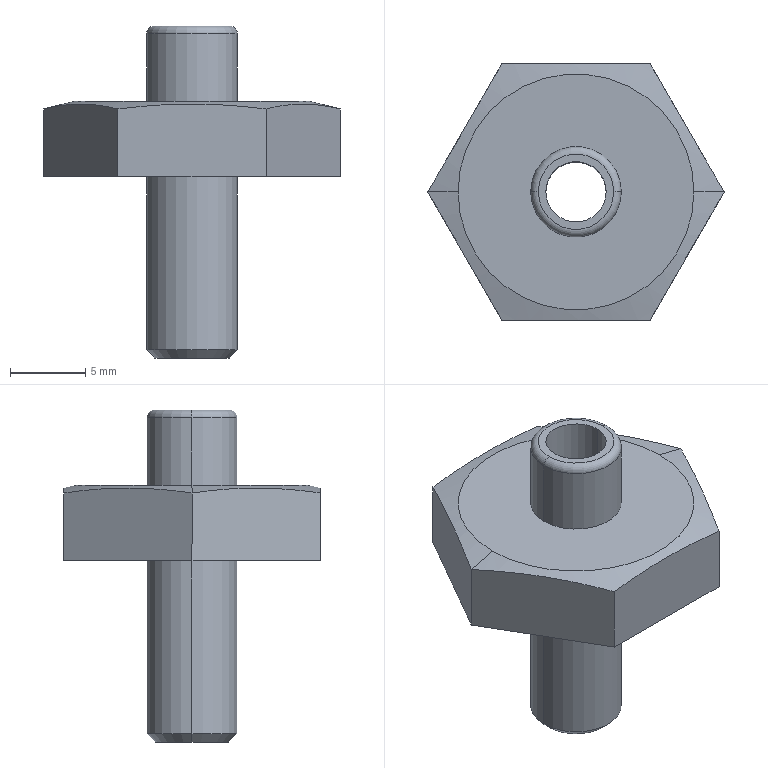Part | SolidWorks | features ICE 2, Cut 1, Extrusion 1, Fillet 1, RevCut 1, StudWizard 1 | 1 solid | 22 faces | box 19.63 x 17 x 22 mm | volume 1443 mm3 | plane 10 | cylinder 6 | cone 4 | torus 2 | commonest cylinder face diameters 6 x4 4 x2
STEP:
#1=CARTESIAN_POINT('',(-119.073,154.119,-12.));
#2=VERTEX_POINT('',#1);
#3=CARTESIAN_POINT('',(-123.99,154.119,-12.));
#4=VERTEX_POINT('',#3);
#5=CARTESIAN_POINT('',(-121.531,154.119,-12.));
#6=DIRECTION('',(0.,0.,1.));
#7=DIRECTION('',(1.,0.,0.));
#8=AXIS2_PLACEMENT_3D('',#5,#6,#7);
#9=CIRCLE('',#8,2.459);
#10=EDGE_CURVE('',#2,#4,#9,.T.);
#11=ORIENTED_EDGE('',*,*,#10,.T.);
#12=CARTESIAN_POINT('',(-124.531,154.119,-11.459));
#13=VERTEX_POINT('',#12);
#14=CARTESIAN_POINT('',(-123.99,154.119,-12.));
#15=DIRECTION('',(-0.7071,0.,0.7071));
#16=VECTOR('',#15,1000.);
#17=LINE('',#14,#16);
#18=EDGE_CURVE('',#4,#13,#17,.T.);
#19=ORIENTED_EDGE('',*,*,#18,.T.);
#20=CARTESIAN_POINT('',(-118.531,154.119,-11.459));
#21=VERTEX_POINT('',#20);
#22=CARTESIAN_POINT('',(-121.531,154.119,-11.459));
#23=DIRECTION('',(0.,0.,1.));
#24=DIRECTION('',(1.,0.,0.));
#25=AXIS2_PLACEMENT_3D('',#22,#23,#24);
#26=CIRCLE('',#25,3.);
#27=EDGE_CURVE('',#21,#13,#26,.T.);
#28=ORIENTED_EDGE('',*,*,#27,.F.);
#29=CARTESIAN_POINT('',(-119.073,154.119,-12.));
#30=DIRECTION('',(0.7071,0.,0.7071));
#31=VECTOR('',#30,1000.);
#32=LINE('',#29,#31);
#33=EDGE_CURVE('',#2,#21,#32,.T.);
#34=ORIENTED_EDGE('',*,*,#33,.F.);
#35=EDGE_LOOP('',(#11,#19,#28,#34));
#36=FACE_OUTER_BOUND('',#35,.T.);
#37=CARTESIAN_POINT('',(-121.531,154.119,-12.));
#38=DIRECTION('',(0.,0.,1.));
#39=DIRECTION('',(1.,0.,0.));
#40=AXIS2_PLACEMENT_3D('',#37,#38,#39);
#41=CONICAL_SURFACE('',#40,2.459,0.7854);
#42=ADVANCED_FACE('',(#36),#41,.T.);
#43=CARTESIAN_POINT('',(-124.531,154.119,9.5));
#44=VERTEX_POINT('',#43);
#45=CARTESIAN_POINT('',(-118.531,154.119,9.5));
#46=VERTEX_POINT('',#45);
#47=CARTESIAN_POINT('',(-121.531,154.119,9.5));
#48=DIRECTION('',(0.,0.,-1.));
#49=DIRECTION('',(1.,0.,0.));
#50=AXIS2_PLACEMENT_3D('',#47,#48,#49);
#51=CIRCLE('',#50,3.);
#52=EDGE_CURVE('',#44,#46,#51,.T.);
#53=ORIENTED_EDGE('',*,*,#52,.F.);
#54=CARTESIAN_POINT('',(-124.031,154.119,10.));
#55=VERTEX_POINT('',#54);
#56=CARTESIAN_POINT('',(-124.031,154.119,9.5));
#57=DIRECTION('',(0.,1.,0.));
#58=DIRECTION('',(-1.,0.,0.));
#59=AXIS2_PLACEMENT_3D('',#56,#57,#58);
#60=CIRCLE('',#59,0.5);
#61=EDGE_CURVE('',#44,#55,#60,.T.);
#62=ORIENTED_EDGE('',*,*,#61,.T.);
#63=CARTESIAN_POINT('',(-119.031,154.119,10.));
#64=VERTEX_POINT('',#63);
#65=CARTESIAN_POINT('',(-121.531,154.119,10.));
#66=DIRECTION('',(0.,0.,1.));
#67=DIRECTION('',(1.,0.,0.));
#68=AXIS2_PLACEMENT_3D('',#65,#66,#67);
#69=CIRCLE('',#68,2.5);
#70=EDGE_CURVE('',#64,#55,#69,.T.);
#71=ORIENTED_EDGE('',*,*,#70,.F.);
#72=CARTESIAN_POINT('',(-119.031,154.119,9.5));
#73=DIRECTION('',(0.,-1.,0.));
#74=DIRECTION('',(0.,0.,-1.));
#75=AXIS2_PLACEMENT_3D('',#72,#73,#74);
#76=CIRCLE('',#75,0.5);
#77=EDGE_CURVE('',#46,#64,#76,.T.);
#78=ORIENTED_EDGE('',*,*,#77,.F.);
#79=EDGE_LOOP('',(#53,#62,#71,#78));
#80=FACE_OUTER_BOUND('',#79,.T.);
#81=CARTESIAN_POINT('',(-121.531,154.119,9.5));
#82=DIRECTION('',(0.,0.,1.));
#83=DIRECTION('',(1.,0.,0.));
#84=AXIS2_PLACEMENT_3D('',#81,#82,#83);
#85=TOROIDAL_SURFACE('',#84,2.5,0.5);
#86=ADVANCED_FACE('',(#80),#85,.T.);
#87=CARTESIAN_POINT('',(-113.716,154.119,5.));
#88=VERTEX_POINT('',#87);
#89=CARTESIAN_POINT('',(-129.346,154.119,5.));
#90=VERTEX_POINT('',#89);
#91=CARTESIAN_POINT('',(-121.531,154.119,5.));
#92=DIRECTION('',(0.,0.,1.));
#93=DIRECTION('',(1.,0.,0.));
#94=AXIS2_PLACEMENT_3D('',#91,#92,#93);
#95=CIRCLE('',#94,7.815);
#96=EDGE_CURVE('',#88,#90,#95,.T.);
#97=ORIENTED_EDGE('',*,*,#96,.F.);
#98=CARTESIAN_POINT('',(-111.716,154.119,4.5));
#99=VERTEX_POINT('',#98);
#100=CARTESIAN_POINT('',(-111.716,154.119,4.5));
#101=DIRECTION('',(0.9701,0.,-0.2425));
#102=VECTOR('',#101,1000.);
#103=LINE('',#100,#102);
#104=EDGE_CURVE('',#88,#99,#103,.T.);
#105=ORIENTED_EDGE('',*,*,#104,.T.);
#106=CARTESIAN_POINT('',(-116.624,162.619,4.5));
#107=VERTEX_POINT('',#106);
#108=CARTESIAN_POINT('',(-116.624,162.619,4.5));
#109=CARTESIAN_POINT('',(-115.806,161.202,4.704));
#110=CARTESIAN_POINT('',(-114.17,158.369,4.953));
#111=CARTESIAN_POINT('',(-112.534,155.536,4.704));
#112=CARTESIAN_POINT('',(-111.716,154.119,4.5));
#113=B_SPLINE_CURVE_WITH_KNOTS('',3,(#108,#109,#110,#111,#112),.UNSPECIFIED.,.F.,.F.,(4,1,4),(0.000000231,0.004908,0.009815),.UNSPECIFIED.);
#114=EDGE_CURVE('',#107,#99,#113,.T.);
#115=ORIENTED_EDGE('',*,*,#114,.F.);
#116=CARTESIAN_POINT('',(-126.439,162.619,4.5));
#117=VERTEX_POINT('',#116);
#118=CARTESIAN_POINT('',(-126.439,162.619,4.5));
#119=CARTESIAN_POINT('',(-124.823,162.619,4.702));
#120=CARTESIAN_POINT('',(-123.199,162.619,4.827));
#121=CARTESIAN_POINT('',(-120.741,162.619,4.829));
#122=CARTESIAN_POINT('',(-119.918,162.619,4.8));
#123=CARTESIAN_POINT('',(-118.265,162.619,4.686));
#124=CARTESIAN_POINT('',(-117.443,162.619,4.602));
#125=CARTESIAN_POINT('',(-116.624,162.619,4.5));
#126=B_SPLINE_CURVE_WITH_KNOTS('',3,(#118,#119,#120,#121,#122,#123,#124,#125),.UNSPECIFIED.,.F.,.F.,(4,2,2,4),(0.009971,0.01485,0.0173,0.01974),.UNSPECIFIED.);
#127=EDGE_CURVE('',#117,#107,#126,.T.);
#128=ORIENTED_EDGE('',*,*,#127,.F.);
#129=CARTESIAN_POINT('',(-131.346,154.119,4.5));
#130=VERTEX_POINT('',#129);
#131=CARTESIAN_POINT('',(-131.346,154.119,4.5));
#132=CARTESIAN_POINT('',(-130.528,155.536,4.704));
#133=CARTESIAN_POINT('',(-128.892,158.369,4.953));
#134=CARTESIAN_POINT('',(-127.257,161.202,4.704));
#135=CARTESIAN_POINT('',(-126.439,162.619,4.5));
#136=B_SPLINE_CURVE_WITH_KNOTS('',3,(#131,#132,#133,#134,#135),.UNSPECIFIED.,.F.,.F.,(4,1,4),(0.000000231,0.004908,0.009815),.UNSPECIFIED.);
#137=EDGE_CURVE('',#130,#117,#136,.T.);
#138=ORIENTED_EDGE('',*,*,#137,.F.);
#139=CARTESIAN_POINT('',(-131.346,154.119,4.5));
#140=DIRECTION('',(-0.9701,0.,-0.2425));
#141=VECTOR('',#140,1000.);
#142=LINE('',#139,#141);
#143=EDGE_CURVE('',#90,#130,#142,.T.);
#144=ORIENTED_EDGE('',*,*,#143,.F.);
#145=EDGE_LOOP('',(#97,#105,#115,#128,#138,#144));
#146=FACE_OUTER_BOUND('',#145,.T.);
#147=CARTESIAN_POINT('',(-121.531,154.119,4.5));
#148=DIRECTION('',(0.,0.,-1.));
#149=DIRECTION('',(-1.,0.,0.));
#150=AXIS2_PLACEMENT_3D('',#147,#148,#149);
#151=CONICAL_SURFACE('',#150,9.815,1.326);
#152=ADVANCED_FACE('',(#146),#151,.T.);
#153=CARTESIAN_POINT('',(-119.531,154.119,-12.));
#154=VERTEX_POINT('',#153);
#155=CARTESIAN_POINT('',(-123.531,154.119,-12.));
#156=VERTEX_POINT('',#155);
#157=CARTESIAN_POINT('',(-121.531,154.119,-12.));
#158=DIRECTION('',(0.,0.,-1.));
#159=DIRECTION('',(-1.,0.,0.));
#160=AXIS2_PLACEMENT_3D('',#157,#158,#159);
#161=CIRCLE('',#160,2.);
#162=EDGE_CURVE('',#154,#156,#161,.T.);
#163=ORIENTED_EDGE('',*,*,#162,.T.);
#164=CARTESIAN_POINT('',(-123.531,154.119,10.));
#165=VERTEX_POINT('',#164);
#166=CARTESIAN_POINT('',(-123.531,154.119,-22.));
#167=DIRECTION('',(0.,0.,1.));
#168=VECTOR('',#167,1000.);
#169=LINE('',#166,#168);
#170=EDGE_CURVE('',#156,#165,#169,.T.);
#171=ORIENTED_EDGE('',*,*,#170,.T.);
#172=CARTESIAN_POINT('',(-119.531,154.119,10.));
#173=VERTEX_POINT('',#172);
#174=CARTESIAN_POINT('',(-121.531,154.119,10.));
#175=DIRECTION('',(0.,0.,1.));
#176=DIRECTION('',(1.,0.,0.));
#177=AXIS2_PLACEMENT_3D('',#174,#175,#176);
#178=CIRCLE('',#177,2.);
#179=EDGE_CURVE('',#165,#173,#178,.T.);
#180=ORIENTED_EDGE('',*,*,#179,.T.);
#181=CARTESIAN_POINT('',(-119.531,154.119,-22.));
#182=DIRECTION('',(0.,0.,1.));
#183=VECTOR('',#182,1000.);
#184=LINE('',#181,#183);
#185=EDGE_CURVE('',#154,#173,#184,.T.);
#186=ORIENTED_EDGE('',*,*,#185,.F.);
#187=EDGE_LOOP('',(#163,#171,#180,#186));
#188=FACE_OUTER_BOUND('',#187,.T.);
#189=CARTESIAN_POINT('',(-121.531,154.119,-22.));
#190=DIRECTION('',(0.,0.,1.));
#191=DIRECTION('',(1.,0.,0.));
#192=AXIS2_PLACEMENT_3D('',#189,#190,#191);
#193=CYLINDRICAL_SURFACE('',#192,2.);
#194=ADVANCED_FACE('',(#188),#193,.F.);
#195=ORIENTED_EDGE('',*,*,#27,.T.);
#196=CARTESIAN_POINT('',(-124.531,154.119,0.));
#197=VERTEX_POINT('',#196);
#198=CARTESIAN_POINT('',(-124.531,154.119,-12.));
#199=DIRECTION('',(0.,0.,1.));
#200=VECTOR('',#199,1000.);
#201=LINE('',#198,#200);
#202=EDGE_CURVE('',#13,#197,#201,.T.);
#203=ORIENTED_EDGE('',*,*,#202,.T.);
#204=CARTESIAN_POINT('',(-118.531,154.119,0.));
#205=VERTEX_POINT('',#204);
#206=CARTESIAN_POINT('',(-121.531,154.119,0.));
#207=DIRECTION('',(0.,0.,-1.));
#208=DIRECTION('',(-1.,0.,0.));
#209=AXIS2_PLACEMENT_3D('',#206,#207,#208);
#210=CIRCLE('',#209,3.);
#211=EDGE_CURVE('',#197,#205,#210,.T.);
#212=ORIENTED_EDGE('',*,*,#211,.T.);
#213=CARTESIAN_POINT('',(-118.531,154.119,-12.));
#214=DIRECTION('',(0.,0.,1.));
#215=VECTOR('',#214,1000.);
#216=LINE('',#213,#215);
#217=EDGE_CURVE('',#21,#205,#216,.T.);
#218=ORIENTED_EDGE('',*,*,#217,.F.);
#219=EDGE_LOOP('',(#195,#203,#212,#218));
#220=FACE_OUTER_BOUND('',#219,.T.);
#221=CARTESIAN_POINT('',(-121.531,154.119,-12.));
#222=DIRECTION('',(0.,0.,1.));
#223=DIRECTION('',(1.,0.,0.));
#224=AXIS2_PLACEMENT_3D('',#221,#222,#223);
#225=CYLINDRICAL_SURFACE('',#224,3.);
#226=ADVANCED_FACE('',(#220),#225,.T.);
#227=ORIENTED_EDGE('',*,*,#52,.T.);
#228=CARTESIAN_POINT('',(-118.531,154.119,5.));
#229=VERTEX_POINT('',#228);
#230=CARTESIAN_POINT('',(-118.531,154.119,10.));
#231=DIRECTION('',(0.,0.,-1.));
#232=VECTOR('',#231,1000.);
#233=LINE('',#230,#232);
#234=EDGE_CURVE('',#46,#229,#233,.T.);
#235=ORIENTED_EDGE('',*,*,#234,.T.);
#236=CARTESIAN_POINT('',(-124.531,154.119,5.));
#237=VERTEX_POINT('',#236);
#238=CARTESIAN_POINT('',(-121.531,154.119,5.));
#239=DIRECTION('',(0.,0.,1.));
#240=DIRECTION('',(1.,0.,0.));
#241=AXIS2_PLACEMENT_3D('',#238,#239,#240);
#242=CIRCLE('',#241,3.);
#243=EDGE_CURVE('',#229,#237,#242,.T.);
#244=ORIENTED_EDGE('',*,*,#243,.T.);
#245=CARTESIAN_POINT('',(-124.531,154.119,10.));
#246=DIRECTION('',(0.,0.,-1.));
#247=VECTOR('',#246,1000.);
#248=LINE('',#245,#247);
#249=EDGE_CURVE('',#44,#237,#248,.T.);
#250=ORIENTED_EDGE('',*,*,#249,.F.);
#251=EDGE_LOOP('',(#227,#235,#244,#250));
#252=FACE_OUTER_BOUND('',#251,.T.);
#253=CARTESIAN_POINT('',(-121.531,154.119,10.));
#254=DIRECTION('',(0.,0.,-1.));
#255=DIRECTION('',(-1.,0.,0.));
#256=AXIS2_PLACEMENT_3D('',#253,#254,#255);
#257=CYLINDRICAL_SURFACE('',#256,3.);
#258=ADVANCED_FACE('',(#252),#257,.T.);
#259=ORIENTED_EDGE('',*,*,#162,.F.);
#260=CARTESIAN_POINT('',(-121.531,154.119,-12.));
#261=DIRECTION('',(0.,0.,-1.));
#262=DIRECTION('',(-1.,0.,0.));
#263=AXIS2_PLACEMENT_3D('',#260,#261,#262);
#264=CIRCLE('',#263,2.);
#265=EDGE_CURVE('',#156,#154,#264,.T.);
#266=ORIENTED_EDGE('',*,*,#265,.F.);
#267=EDGE_LOOP('',(#259,#266));
#268=FACE_BOUND('',#267,.T.);
#269=ORIENTED_EDGE('',*,*,#10,.F.);
#270=CARTESIAN_POINT('',(-121.531,154.119,-12.));
#271=DIRECTION('',(0.,0.,1.));
#272=DIRECTION('',(1.,0.,0.));
#273=AXIS2_PLACEMENT_3D('',#270,#271,#272);
#274=CIRCLE('',#273,2.459);
#275=EDGE_CURVE('',#4,#2,#274,.T.);
#276=ORIENTED_EDGE('',*,*,#275,.F.);
#277=EDGE_LOOP('',(#269,#276));
#278=FACE_OUTER_BOUND('',#277,.T.);
#279=CARTESIAN_POINT('',(-121.531,154.119,-12.));
#280=DIRECTION('',(0.,0.,-1.));
#281=DIRECTION('',(-1.,0.,0.));
#282=AXIS2_PLACEMENT_3D('',#279,#280,#281);
#283=PLANE('',#282);
#284=ADVANCED_FACE('',(#268,#278),#283,.T.);
#285=CARTESIAN_POINT('',(-121.531,154.119,5.));
#286=DIRECTION('',(0.,0.,1.));
#287=DIRECTION('',(1.,0.,0.));
#288=AXIS2_PLACEMENT_3D('',#285,#286,#287);
#289=CIRCLE('',#288,3.);
#290=EDGE_CURVE('',#237,#229,#289,.T.);
#291=ORIENTED_EDGE('',*,*,#290,.F.);
#292=ORIENTED_EDGE('',*,*,#243,.F.);
#293=EDGE_LOOP('',(#291,#292));
#294=FACE_BOUND('',#293,.T.);
#295=CARTESIAN_POINT('',(-121.531,154.119,5.));
#296=DIRECTION('',(0.,0.,1.));
#297=DIRECTION('',(1.,0.,0.));
#298=AXIS2_PLACEMENT_3D('',#295,#296,#297);
#299=CIRCLE('',#298,7.815);
#300=EDGE_CURVE('',#90,#88,#299,.T.);
#301=ORIENTED_EDGE('',*,*,#300,.T.);
#302=ORIENTED_EDGE('',*,*,#96,.T.);
#303=EDGE_LOOP('',(#301,#302));
#304=FACE_OUTER_BOUND('',#303,.T.);
#305=CARTESIAN_POINT('',(0.,0.,5.));
#306=DIRECTION('',(0.,0.,1.));
#307=DIRECTION('',(1.,0.,0.));
#308=AXIS2_PLACEMENT_3D('',#305,#306,#307);
#309=PLANE('',#308);
#310=ADVANCED_FACE('',(#294,#304),#309,.T.);
#311=CARTESIAN_POINT('',(-116.624,162.619,0.));
#312=VERTEX_POINT('',#311);
#313=CARTESIAN_POINT('',(-116.624,162.619,5.));
#314=DIRECTION('',(0.,0.,-1.));
#315=VECTOR('',#314,1000.);
#316=LINE('',#313,#315);
#317=EDGE_CURVE('',#107,#312,#316,.T.);
#318=ORIENTED_EDGE('',*,*,#317,.F.);
#319=ORIENTED_EDGE('',*,*,#114,.T.);
#320=CARTESIAN_POINT('',(-111.716,154.119,0.));
#321=VERTEX_POINT('',#320);
#322=CARTESIAN_POINT('',(-111.716,154.119,5.));
#323=DIRECTION('',(0.,0.,-1.));
#324=VECTOR('',#323,1000.);
#325=LINE('',#322,#324);
#326=EDGE_CURVE('',#99,#321,#325,.T.);
#327=ORIENTED_EDGE('',*,*,#326,.T.);
#328=CARTESIAN_POINT('',(-111.716,154.119,0.));
#329=DIRECTION('',(-0.5,0.866,0.));
#330=VECTOR('',#329,1000.);
#331=LINE('',#328,#330);
#332=EDGE_CURVE('',#321,#312,#331,.T.);
#333=ORIENTED_EDGE('',*,*,#332,.T.);
#334=EDGE_LOOP('',(#318,#319,#327,#333));
#335=FACE_OUTER_BOUND('',#334,.T.);
#336=CARTESIAN_POINT('',(-111.716,154.119,5.));
#337=DIRECTION('',(-0.866,-0.5,0.));
#338=DIRECTION('',(0.5,-0.866,0.));
#339=AXIS2_PLACEMENT_3D('',#336,#337,#338);
#340=PLANE('',#339);
#341=ADVANCED_FACE('',(#335),#340,.F.);
#342=CARTESIAN_POINT('',(-126.439,162.619,0.));
#343=VERTEX_POINT('',#342);
#344=CARTESIAN_POINT('',(-126.439,162.619,5.));
#345=DIRECTION('',(0.,0.,-1.));
#346=VECTOR('',#345,1000.);
#347=LINE('',#344,#346);
#348=EDGE_CURVE('',#117,#343,#347,.T.);
#349=ORIENTED_EDGE('',*,*,#348,.F.);
#350=ORIENTED_EDGE('',*,*,#127,.T.);
#351=ORIENTED_EDGE('',*,*,#317,.T.);
#352=CARTESIAN_POINT('',(-116.624,162.619,0.));
#353=DIRECTION('',(-1.,0.,0.));
#354=VECTOR('',#353,1000.);
#355=LINE('',#352,#354);
#356=EDGE_CURVE('',#312,#343,#355,.T.);
#357=ORIENTED_EDGE('',*,*,#356,.T.);
#358=EDGE_LOOP('',(#349,#350,#351,#357));
#359=FACE_OUTER_BOUND('',#358,.T.);
#360=CARTESIAN_POINT('',(-116.624,162.619,5.));
#361=DIRECTION('',(0.,-1.,0.));
#362=DIRECTION('',(0.,0.,-1.));
#363=AXIS2_PLACEMENT_3D('',#360,#361,#362);
#364=PLANE('',#363);
#365=ADVANCED_FACE('',(#359),#364,.F.);
#366=CARTESIAN_POINT('',(-131.346,154.119,0.));
#367=VERTEX_POINT('',#366);
#368=CARTESIAN_POINT('',(-131.346,154.119,5.));
#369=DIRECTION('',(0.,0.,-1.));
#370=VECTOR('',#369,1000.);
#371=LINE('',#368,#370);
#372=EDGE_CURVE('',#130,#367,#371,.T.);
#373=ORIENTED_EDGE('',*,*,#372,.F.);
#374=ORIENTED_EDGE('',*,*,#137,.T.);
#375=ORIENTED_EDGE('',*,*,#348,.T.);
#376=CARTESIAN_POINT('',(-126.439,162.619,0.));
#377=DIRECTION('',(-0.5,-0.866,0.));
#378=VECTOR('',#377,1000.);
#379=LINE('',#376,#378);
#380=EDGE_CURVE('',#343,#367,#379,.T.);
#381=ORIENTED_EDGE('',*,*,#380,.T.);
#382=EDGE_LOOP('',(#373,#374,#375,#381));
#383=FACE_OUTER_BOUND('',#382,.T.);
#384=CARTESIAN_POINT('',(-126.439,162.619,5.));
#385=DIRECTION('',(0.866,-0.5,0.));
#386=DIRECTION('',(0.5,0.866,0.));
#387=AXIS2_PLACEMENT_3D('',#384,#385,#386);
#388=PLANE('',#387);
#389=ADVANCED_FACE('',(#383),#388,.F.);
#390=CARTESIAN_POINT('',(-126.439,145.619,4.5));
#391=VERTEX_POINT('',#390);
#392=CARTESIAN_POINT('',(-126.439,145.619,0.));
#393=VERTEX_POINT('',#392);
#394=CARTESIAN_POINT('',(-126.439,145.619,5.));
#395=DIRECTION('',(0.,0.,-1.));
#396=VECTOR('',#395,1000.);
#397=LINE('',#394,#396);
#398=EDGE_CURVE('',#391,#393,#397,.T.);
#399=ORIENTED_EDGE('',*,*,#398,.F.);
#400=CARTESIAN_POINT('',(-126.439,145.619,4.5));
#401=CARTESIAN_POINT('',(-127.257,147.036,4.704));
#402=CARTESIAN_POINT('',(-128.892,149.869,4.953));
#403=CARTESIAN_POINT('',(-130.528,152.702,4.704));
#404=CARTESIAN_POINT('',(-131.346,154.119,4.5));
#405=B_SPLINE_CURVE_WITH_KNOTS('',3,(#400,#401,#402,#403,#404),.UNSPECIFIED.,.F.,.F.,(4,1,4),(0.000000231,0.004908,0.009815),.UNSPECIFIED.);
#406=EDGE_CURVE('',#391,#130,#405,.T.);
#407=ORIENTED_EDGE('',*,*,#406,.T.);
#408=ORIENTED_EDGE('',*,*,#372,.T.);
#409=CARTESIAN_POINT('',(-131.346,154.119,0.));
#410=DIRECTION('',(0.5,-0.866,0.));
#411=VECTOR('',#410,1000.);
#412=LINE('',#409,#411);
#413=EDGE_CURVE('',#367,#393,#412,.T.);
#414=ORIENTED_EDGE('',*,*,#413,.T.);
#415=EDGE_LOOP('',(#399,#407,#408,#414));
#416=FACE_OUTER_BOUND('',#415,.T.);
#417=CARTESIAN_POINT('',(-131.346,154.119,5.));
#418=DIRECTION('',(0.866,0.5,0.));
#419=DIRECTION('',(-0.5,0.866,0.));
#420=AXIS2_PLACEMENT_3D('',#417,#418,#419);
#421=PLANE('',#420);
#422=ADVANCED_FACE('',(#416),#421,.F.);
#423=CARTESIAN_POINT('',(-116.624,145.619,4.5));
#424=VERTEX_POINT('',#423);
#425=CARTESIAN_POINT('',(-116.624,145.619,0.));
#426=VERTEX_POINT('',#425);
#427=CARTESIAN_POINT('',(-116.624,145.619,5.));
#428=DIRECTION('',(0.,0.,-1.));
#429=VECTOR('',#428,1000.);
#430=LINE('',#427,#429);
#431=EDGE_CURVE('',#424,#426,#430,.T.);
#432=ORIENTED_EDGE('',*,*,#431,.F.);
#433=CARTESIAN_POINT('',(-116.624,145.619,4.5));
#434=CARTESIAN_POINT('',(-118.239,145.619,4.702));
#435=CARTESIAN_POINT('',(-119.863,145.619,4.827));
#436=CARTESIAN_POINT('',(-122.321,145.619,4.829));
#437=CARTESIAN_POINT('',(-123.145,145.619,4.8));
#438=CARTESIAN_POINT('',(-124.797,145.619,4.686));
#439=CARTESIAN_POINT('',(-125.62,145.619,4.602));
#440=CARTESIAN_POINT('',(-126.439,145.619,4.5));
#441=B_SPLINE_CURVE_WITH_KNOTS('',3,(#433,#434,#435,#436,#437,#438,#439,#440),.UNSPECIFIED.,.F.,.F.,(4,2,2,4),(0.009971,0.01485,0.0173,0.01974),.UNSPECIFIED.);
#442=EDGE_CURVE('',#424,#391,#441,.T.);
#443=ORIENTED_EDGE('',*,*,#442,.T.);
#444=ORIENTED_EDGE('',*,*,#398,.T.);
#445=CARTESIAN_POINT('',(-126.439,145.619,0.));
#446=DIRECTION('',(1.,0.,0.));
#447=VECTOR('',#446,1000.);
#448=LINE('',#445,#447);
#449=EDGE_CURVE('',#393,#426,#448,.T.);
#450=ORIENTED_EDGE('',*,*,#449,.T.);
#451=EDGE_LOOP('',(#432,#443,#444,#450));
#452=FACE_OUTER_BOUND('',#451,.T.);
#453=CARTESIAN_POINT('',(-126.439,145.619,5.));
#454=DIRECTION('',(0.,1.,0.));
#455=DIRECTION('',(0.,0.,1.));
#456=AXIS2_PLACEMENT_3D('',#453,#454,#455);
#457=PLANE('',#456);
#458=ADVANCED_FACE('',(#452),#457,.F.);
#459=ORIENTED_EDGE('',*,*,#326,.F.);
#460=CARTESIAN_POINT('',(-111.716,154.119,4.5));
#461=CARTESIAN_POINT('',(-112.534,152.702,4.704));
#462=CARTESIAN_POINT('',(-114.17,149.869,4.953));
#463=CARTESIAN_POINT('',(-115.806,147.036,4.704));
#464=CARTESIAN_POINT('',(-116.624,145.619,4.5));
#465=B_SPLINE_CURVE_WITH_KNOTS('',3,(#460,#461,#462,#463,#464),.UNSPECIFIED.,.F.,.F.,(4,1,4),(0.000000231,0.004908,0.009815),.UNSPECIFIED.);
#466=EDGE_CURVE('',#99,#424,#465,.T.);
#467=ORIENTED_EDGE('',*,*,#466,.T.);
#468=ORIENTED_EDGE('',*,*,#431,.T.);
#469=CARTESIAN_POINT('',(-116.624,145.619,0.));
#470=DIRECTION('',(0.5,0.866,0.));
#471=VECTOR('',#470,1000.);
#472=LINE('',#469,#471);
#473=EDGE_CURVE('',#426,#321,#472,.T.);
#474=ORIENTED_EDGE('',*,*,#473,.T.);
#475=EDGE_LOOP('',(#459,#467,#468,#474));
#476=FACE_OUTER_BOUND('',#475,.T.);
#477=CARTESIAN_POINT('',(-116.624,145.619,5.));
#478=DIRECTION('',(-0.866,0.5,0.));
#479=DIRECTION('',(-0.5,-0.866,0.));
#480=AXIS2_PLACEMENT_3D('',#477,#478,#479);
#481=PLANE('',#480);
#482=ADVANCED_FACE('',(#476),#481,.F.);
#483=CARTESIAN_POINT('',(-121.531,154.119,0.));
#484=DIRECTION('',(0.,0.,-1.));
#485=DIRECTION('',(-1.,0.,0.));
#486=AXIS2_PLACEMENT_3D('',#483,#484,#485);
#487=CIRCLE('',#486,3.);
#488=EDGE_CURVE('',#205,#197,#487,.T.);
#489=ORIENTED_EDGE('',*,*,#488,.F.);
#490=ORIENTED_EDGE('',*,*,#211,.F.);
#491=EDGE_LOOP('',(#489,#490));
#492=FACE_BOUND('',#491,.T.);
#493=ORIENTED_EDGE('',*,*,#332,.F.);
#494=ORIENTED_EDGE('',*,*,#473,.F.);
#495=ORIENTED_EDGE('',*,*,#449,.F.);
#496=ORIENTED_EDGE('',*,*,#413,.F.);
#497=ORIENTED_EDGE('',*,*,#380,.F.);
#498=ORIENTED_EDGE('',*,*,#356,.F.);
#499=EDGE_LOOP('',(#493,#494,#495,#496,#497,#498));
#500=FACE_OUTER_BOUND('',#499,.T.);
#501=CARTESIAN_POINT('',(0.,0.,0.));
#502=DIRECTION('',(0.,0.,1.));
#503=DIRECTION('',(1.,0.,0.));
#504=AXIS2_PLACEMENT_3D('',#501,#502,#503);
#505=PLANE('',#504);
#506=ADVANCED_FACE('',(#492,#500),#505,.F.);
#507=ORIENTED_EDGE('',*,*,#234,.F.);
#508=CARTESIAN_POINT('',(-121.531,154.119,9.5));
#509=DIRECTION('',(0.,0.,-1.));
#510=DIRECTION('',(1.,0.,0.));
#511=AXIS2_PLACEMENT_3D('',#508,#509,#510);
#512=CIRCLE('',#511,3.);
#513=EDGE_CURVE('',#46,#44,#512,.T.);
#514=ORIENTED_EDGE('',*,*,#513,.T.);
#515=ORIENTED_EDGE('',*,*,#249,.T.);
#516=ORIENTED_EDGE('',*,*,#290,.T.);
#517=EDGE_LOOP('',(#507,#514,#515,#516));
#518=FACE_OUTER_BOUND('',#517,.T.);
#519=CARTESIAN_POINT('',(-121.531,154.119,10.));
#520=DIRECTION('',(0.,0.,-1.));
#521=DIRECTION('',(-1.,0.,0.));
#522=AXIS2_PLACEMENT_3D('',#519,#520,#521);
#523=CYLINDRICAL_SURFACE('',#522,3.);
#524=ADVANCED_FACE('',(#518),#523,.T.);
#525=ORIENTED_EDGE('',*,*,#70,.T.);
#526=CARTESIAN_POINT('',(-121.531,154.119,10.));
#527=DIRECTION('',(0.,0.,1.));
#528=DIRECTION('',(1.,0.,0.));
#529=AXIS2_PLACEMENT_3D('',#526,#527,#528);
#530=CIRCLE('',#529,2.5);
#531=EDGE_CURVE('',#55,#64,#530,.T.);
#532=ORIENTED_EDGE('',*,*,#531,.T.);
#533=EDGE_LOOP('',(#525,#532));
#534=FACE_OUTER_BOUND('',#533,.T.);
#535=CARTESIAN_POINT('',(-121.531,154.119,10.));
#536=DIRECTION('',(0.,0.,1.));
#537=DIRECTION('',(1.,0.,0.));
#538=AXIS2_PLACEMENT_3D('',#535,#536,#537);
#539=CIRCLE('',#538,2.);
#540=EDGE_CURVE('',#173,#165,#539,.T.);
#541=ORIENTED_EDGE('',*,*,#540,.F.);
#542=ORIENTED_EDGE('',*,*,#179,.F.);
#543=EDGE_LOOP('',(#541,#542));
#544=FACE_BOUND('',#543,.T.);
#545=CARTESIAN_POINT('',(-121.531,154.119,10.));
#546=DIRECTION('',(0.,0.,1.));
#547=DIRECTION('',(1.,0.,0.));
#548=AXIS2_PLACEMENT_3D('',#545,#546,#547);
#549=PLANE('',#548);
#550=ADVANCED_FACE('',(#534,#544),#549,.T.);
#551=ORIENTED_EDGE('',*,*,#202,.F.);
#552=CARTESIAN_POINT('',(-121.531,154.119,-11.459));
#553=DIRECTION('',(0.,0.,1.));
#554=DIRECTION('',(1.,0.,0.));
#555=AXIS2_PLACEMENT_3D('',#552,#553,#554);
#556=CIRCLE('',#555,3.);
#557=EDGE_CURVE('',#13,#21,#556,.T.);
#558=ORIENTED_EDGE('',*,*,#557,.T.);
#559=ORIENTED_EDGE('',*,*,#217,.T.);
#560=ORIENTED_EDGE('',*,*,#488,.T.);
#561=EDGE_LOOP('',(#551,#558,#559,#560));
#562=FACE_OUTER_BOUND('',#561,.T.);
#563=CARTESIAN_POINT('',(-121.531,154.119,-12.));
#564=DIRECTION('',(0.,0.,1.));
#565=DIRECTION('',(1.,0.,0.));
#566=AXIS2_PLACEMENT_3D('',#563,#564,#565);
#567=CYLINDRICAL_SURFACE('',#566,3.);
#568=ADVANCED_FACE('',(#562),#567,.T.);
#569=ORIENTED_EDGE('',*,*,#170,.F.);
#570=ORIENTED_EDGE('',*,*,#265,.T.);
#571=ORIENTED_EDGE('',*,*,#185,.T.);
#572=ORIENTED_EDGE('',*,*,#540,.T.);
#573=EDGE_LOOP('',(#569,#570,#571,#572));
#574=FACE_OUTER_BOUND('',#573,.T.);
#575=CARTESIAN_POINT('',(-121.531,154.119,-22.));
#576=DIRECTION('',(0.,0.,1.));
#577=DIRECTION('',(1.,0.,0.));
#578=AXIS2_PLACEMENT_3D('',#575,#576,#577);
#579=CYLINDRICAL_SURFACE('',#578,2.);
#580=ADVANCED_FACE('',(#574),#579,.F.);
#581=ORIENTED_EDGE('',*,*,#104,.F.);
#582=ORIENTED_EDGE('',*,*,#300,.F.);
#583=ORIENTED_EDGE('',*,*,#143,.T.);
#584=ORIENTED_EDGE('',*,*,#406,.F.);
#585=ORIENTED_EDGE('',*,*,#442,.F.);
#586=ORIENTED_EDGE('',*,*,#466,.F.);
#587=EDGE_LOOP('',(#581,#582,#583,#584,#585,#586));
#588=FACE_OUTER_BOUND('',#587,.T.);
#589=CARTESIAN_POINT('',(-121.531,154.119,4.5));
#590=DIRECTION('',(0.,0.,-1.));
#591=DIRECTION('',(-1.,0.,0.));
#592=AXIS2_PLACEMENT_3D('',#589,#590,#591);
#593=CONICAL_SURFACE('',#592,9.815,1.326);
#594=ADVANCED_FACE('',(#588),#593,.T.);
#595=ORIENTED_EDGE('',*,*,#61,.F.);
#596=ORIENTED_EDGE('',*,*,#513,.F.);
#597=ORIENTED_EDGE('',*,*,#77,.T.);
#598=ORIENTED_EDGE('',*,*,#531,.F.);
#599=EDGE_LOOP('',(#595,#596,#597,#598));
#600=FACE_OUTER_BOUND('',#599,.T.);
#601=CARTESIAN_POINT('',(-121.531,154.119,9.5));
#602=DIRECTION('',(0.,0.,1.));
#603=DIRECTION('',(1.,0.,0.));
#604=AXIS2_PLACEMENT_3D('',#601,#602,#603);
#605=TOROIDAL_SURFACE('',#604,2.5,0.5);
#606=ADVANCED_FACE('',(#600),#605,.T.);
#607=ORIENTED_EDGE('',*,*,#18,.F.);
#608=ORIENTED_EDGE('',*,*,#275,.T.);
#609=ORIENTED_EDGE('',*,*,#33,.T.);
#610=ORIENTED_EDGE('',*,*,#557,.F.);
#611=EDGE_LOOP('',(#607,#608,#609,#610));
#612=FACE_OUTER_BOUND('',#611,.T.);
#613=CARTESIAN_POINT('',(-121.531,154.119,-12.));
#614=DIRECTION('',(0.,0.,1.));
#615=DIRECTION('',(1.,0.,0.));
#616=AXIS2_PLACEMENT_3D('',#613,#614,#615);
#617=CONICAL_SURFACE('',#616,2.459,0.7854);
#618=ADVANCED_FACE('',(#612),#617,.T.);
#619=CLOSED_SHELL('',(#42,#86,#152,#194,#226,#258,#284,#310,#341,#365,#389,#422,#458,#482,#506,#524,#550,#568,#580,#594,#606,#618));
#620=MANIFOLD_SOLID_BREP('',#619);
#621=CARTESIAN_POINT('',(0.,0.,0.));
#622=DIRECTION('',(0.,0.,1.));
#623=DIRECTION('',(1.,0.,0.));
#624=AXIS2_PLACEMENT_3D('',#621,#622,#623);
#625=(LENGTH_UNIT()NAMED_UNIT(*)SI_UNIT(.MILLI.,.METRE.));
#626=UNCERTAINTY_MEASURE_WITH_UNIT(LENGTH_MEASURE(0.00001),#625,'','');
#627=(NAMED_UNIT(*)PLANE_ANGLE_UNIT()SI_UNIT($,.RADIAN.));
#628=(NAMED_UNIT(*)SI_UNIT($,.STERADIAN.)SOLID_ANGLE_UNIT());
#629=(GEOMETRIC_REPRESENTATION_CONTEXT(3)GLOBAL_UNCERTAINTY_ASSIGNED_CONTEXT((#626))GLOBAL_UNIT_ASSIGNED_CONTEXT((#625,#627,#628))REPRESENTATION_CONTEXT('',''));
#630=ADVANCED_BREP_SHAPE_REPRESENTATION('',(#620,#624),#629);